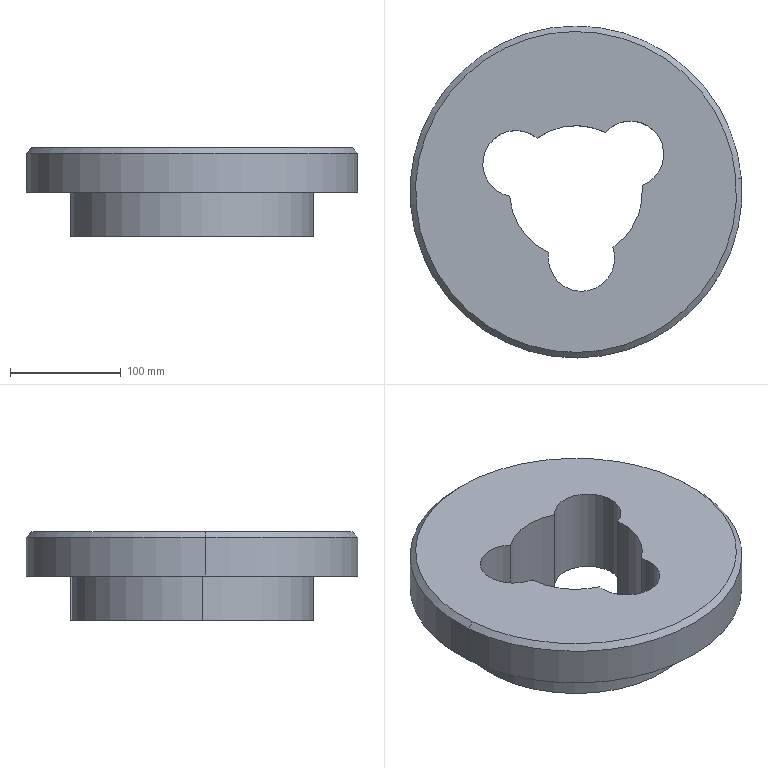Part | SolidWorks | features BaseBody 1 | 1 solid | 25 faces | box 300 x 300 x 80 mm | volume 3048135 mm3 | cylinder 17 | plane 6 | cone 2 | commonest cylinder face diameters 60 x7 120 x5 220 x3 300 x2
STEP:
#1=CARTESIAN_POINT('',(120.577,941.215,-684.893));
#2=VERTEX_POINT('',#1);
#3=CARTESIAN_POINT('',(115.594,940.8,-689.893));
#4=VERTEX_POINT('',#3);
#5=CARTESIAN_POINT('',(115.594,940.8,-689.893));
#6=DIRECTION('',(-0.7047,-0.05869,-0.7071));
#7=VECTOR('',#6,1000.);
#8=LINE('',#5,#7);
#9=EDGE_CURVE('',#2,#4,#8,.T.);
#10=ORIENTED_EDGE('',*,*,#9,.F.);
#11=CARTESIAN_POINT('',(409.577,965.283,-684.893));
#12=VERTEX_POINT('',#11);
#13=CARTESIAN_POINT('',(265.077,953.249,-684.893));
#14=DIRECTION('',(0.,0.,1.));
#15=DIRECTION('',(0.9965,0.083,0.));
#16=AXIS2_PLACEMENT_3D('',#13,#14,#15);
#17=CIRCLE('',#16,145.);
#18=EDGE_CURVE('',#12,#2,#17,.T.);
#19=ORIENTED_EDGE('',*,*,#18,.F.);
#20=CARTESIAN_POINT('',(414.559,965.698,-689.893));
#21=VERTEX_POINT('',#20);
#22=CARTESIAN_POINT('',(414.559,965.698,-689.893));
#23=DIRECTION('',(0.7047,0.05869,-0.7071));
#24=VECTOR('',#23,1000.);
#25=LINE('',#22,#24);
#26=EDGE_CURVE('',#12,#21,#25,.T.);
#27=ORIENTED_EDGE('',*,*,#26,.T.);
#28=CARTESIAN_POINT('',(265.077,953.249,-689.893));
#29=DIRECTION('',(0.,0.,-1.));
#30=DIRECTION('',(0.9965,0.083,0.));
#31=AXIS2_PLACEMENT_3D('',#28,#29,#30);
#32=CIRCLE('',#31,150.);
#33=EDGE_CURVE('',#4,#21,#32,.T.);
#34=ORIENTED_EDGE('',*,*,#33,.F.);
#35=EDGE_LOOP('',(#10,#19,#27,#34));
#36=FACE_OUTER_BOUND('',#35,.T.);
#37=CARTESIAN_POINT('',(265.077,953.249,-689.893));
#38=DIRECTION('',(0.,0.,-1.));
#39=DIRECTION('',(-0.9965,-0.083,0.));
#40=AXIS2_PLACEMENT_3D('',#37,#38,#39);
#41=CONICAL_SURFACE('',#40,150.,0.7854);
#42=ADVANCED_FACE('',(#36),#41,.T.);
#43=CARTESIAN_POINT('',(265.951,1063.245,-724.893));
#44=VERTEX_POINT('',#43);
#45=CARTESIAN_POINT('',(374.697,962.379,-724.893));
#46=VERTEX_POINT('',#45);
#47=CARTESIAN_POINT('',(265.077,953.249,-724.893));
#48=DIRECTION('',(0.,0.,-1.));
#49=DIRECTION('',(0.9965,0.083,0.));
#50=AXIS2_PLACEMENT_3D('',#47,#48,#49);
#51=CIRCLE('',#50,110.);
#52=EDGE_CURVE('',#44,#46,#51,.T.);
#53=ORIENTED_EDGE('',*,*,#52,.F.);
#54=CARTESIAN_POINT('',(266.743,1053.734,-724.893));
#55=VERTEX_POINT('',#54);
#56=CARTESIAN_POINT('',(247.642,1283.081,-724.893));
#57=DIRECTION('',(0.083,-0.9965,0.));
#58=VECTOR('',#57,1000.);
#59=LINE('',#56,#58);
#60=EDGE_CURVE('',#44,#55,#59,.T.);
#61=ORIENTED_EDGE('',*,*,#60,.T.);
#62=CARTESIAN_POINT('',(246.812,1052.074,-724.893));
#63=VERTEX_POINT('',#62);
#64=CARTESIAN_POINT('',(256.777,1052.904,-724.893));
#65=DIRECTION('',(0.9965,0.083,0.));
#66=VECTOR('',#65,1000.);
#67=LINE('',#64,#66);
#68=EDGE_CURVE('',#63,#55,#67,.T.);
#69=ORIENTED_EDGE('',*,*,#68,.F.);
#70=CARTESIAN_POINT('',(246.02,1061.586,-724.893));
#71=VERTEX_POINT('',#70);
#72=CARTESIAN_POINT('',(227.711,1281.421,-724.893));
#73=DIRECTION('',(0.083,-0.9965,0.));
#74=VECTOR('',#73,1000.);
#75=LINE('',#72,#74);
#76=EDGE_CURVE('',#71,#63,#75,.T.);
#77=ORIENTED_EDGE('',*,*,#76,.F.);
#78=CARTESIAN_POINT('',(155.456,944.119,-724.893));
#79=VERTEX_POINT('',#78);
#80=CARTESIAN_POINT('',(265.077,953.249,-724.893));
#81=DIRECTION('',(0.,0.,-1.));
#82=DIRECTION('',(0.9965,0.083,0.));
#83=AXIS2_PLACEMENT_3D('',#80,#81,#82);
#84=CIRCLE('',#83,110.);
#85=EDGE_CURVE('',#79,#71,#84,.T.);
#86=ORIENTED_EDGE('',*,*,#85,.F.);
#87=CARTESIAN_POINT('',(265.077,953.249,-724.893));
#88=DIRECTION('',(0.,0.,-1.));
#89=DIRECTION('',(0.9965,0.083,0.));
#90=AXIS2_PLACEMENT_3D('',#87,#88,#89);
#91=CIRCLE('',#90,110.);
#92=EDGE_CURVE('',#46,#79,#91,.T.);
#93=ORIENTED_EDGE('',*,*,#92,.F.);
#94=EDGE_LOOP('',(#53,#61,#69,#77,#86,#93));
#95=FACE_BOUND('',#94,.T.);
#96=CARTESIAN_POINT('',(414.559,965.698,-724.893));
#97=VERTEX_POINT('',#96);
#98=CARTESIAN_POINT('',(115.594,940.8,-724.893));
#99=VERTEX_POINT('',#98);
#100=CARTESIAN_POINT('',(265.077,953.249,-724.893));
#101=DIRECTION('',(0.,0.,-1.));
#102=DIRECTION('',(0.9965,0.083,0.));
#103=AXIS2_PLACEMENT_3D('',#100,#101,#102);
#104=CIRCLE('',#103,150.);
#105=EDGE_CURVE('',#97,#99,#104,.T.);
#106=ORIENTED_EDGE('',*,*,#105,.T.);
#107=CARTESIAN_POINT('',(265.077,953.249,-724.893));
#108=DIRECTION('',(0.,0.,-1.));
#109=DIRECTION('',(0.9965,0.083,0.));
#110=AXIS2_PLACEMENT_3D('',#107,#108,#109);
#111=CIRCLE('',#110,150.);
#112=EDGE_CURVE('',#99,#97,#111,.T.);
#113=ORIENTED_EDGE('',*,*,#112,.T.);
#114=EDGE_LOOP('',(#106,#113));
#115=FACE_OUTER_BOUND('',#114,.T.);
#116=CARTESIAN_POINT('',(237.676,1282.251,-724.893));
#117=DIRECTION('',(0.,0.,-1.));
#118=DIRECTION('',(0.,-1.,0.));
#119=AXIS2_PLACEMENT_3D('',#116,#117,#118);
#120=PLANE('',#119);
#121=ADVANCED_FACE('',(#95,#115),#120,.T.);
#122=CARTESIAN_POINT('',(324.769,959.318,-684.893));
#123=VERTEX_POINT('',#122);
#124=CARTESIAN_POINT('',(324.87,958.229,-684.893));
#125=VERTEX_POINT('',#124);
#126=CARTESIAN_POINT('',(265.077,953.249,-684.893));
#127=DIRECTION('',(0.,0.,-1.));
#128=DIRECTION('',(0.9965,0.083,0.));
#129=AXIS2_PLACEMENT_3D('',#126,#127,#128);
#130=CIRCLE('',#129,60.);
#131=EDGE_CURVE('',#123,#125,#130,.T.);
#132=ORIENTED_EDGE('',*,*,#131,.T.);
#133=CARTESIAN_POINT('',(298.381,903.341,-684.893));
#134=VERTEX_POINT('',#133);
#135=CARTESIAN_POINT('',(265.077,953.249,-684.893));
#136=DIRECTION('',(0.,0.,-1.));
#137=DIRECTION('',(0.9965,0.083,0.));
#138=AXIS2_PLACEMENT_3D('',#135,#136,#137);
#139=CIRCLE('',#138,60.);
#140=EDGE_CURVE('',#125,#134,#139,.T.);
#141=ORIENTED_EDGE('',*,*,#140,.T.);
#142=CARTESIAN_POINT('',(299.953,895.946,-684.893));
#143=VERTEX_POINT('',#142);
#144=CARTESIAN_POINT('',(270.057,893.456,-684.893));
#145=DIRECTION('',(0.,0.,-1.));
#146=DIRECTION('',(0.9965,0.083,0.));
#147=AXIS2_PLACEMENT_3D('',#144,#145,#146);
#148=CIRCLE('',#147,30.);
#149=EDGE_CURVE('',#134,#143,#148,.T.);
#150=ORIENTED_EDGE('',*,*,#149,.T.);
#151=CARTESIAN_POINT('',(240.16,890.966,-684.893));
#152=VERTEX_POINT('',#151);
#153=CARTESIAN_POINT('',(270.057,893.456,-684.893));
#154=DIRECTION('',(0.,0.,-1.));
#155=DIRECTION('',(0.9965,0.083,0.));
#156=AXIS2_PLACEMENT_3D('',#153,#154,#155);
#157=CIRCLE('',#156,30.);
#158=EDGE_CURVE('',#143,#152,#157,.T.);
#159=ORIENTED_EDGE('',*,*,#158,.T.);
#160=CARTESIAN_POINT('',(240.487,898.519,-684.893));
#161=VERTEX_POINT('',#160);
#162=CARTESIAN_POINT('',(270.057,893.456,-684.893));
#163=DIRECTION('',(0.,0.,-1.));
#164=DIRECTION('',(0.9965,0.083,0.));
#165=AXIS2_PLACEMENT_3D('',#162,#163,#164);
#166=CIRCLE('',#165,30.);
#167=EDGE_CURVE('',#152,#161,#166,.T.);
#168=ORIENTED_EDGE('',*,*,#167,.T.);
#169=CARTESIAN_POINT('',(205.284,948.269,-684.893));
#170=VERTEX_POINT('',#169);
#171=CARTESIAN_POINT('',(265.077,953.249,-684.893));
#172=DIRECTION('',(0.,0.,-1.));
#173=DIRECTION('',(0.9965,0.083,0.));
#174=AXIS2_PLACEMENT_3D('',#171,#172,#173);
#175=CIRCLE('',#174,60.);
#176=EDGE_CURVE('',#161,#170,#175,.T.);
#177=ORIENTED_EDGE('',*,*,#176,.T.);
#178=CARTESIAN_POINT('',(205.203,949.36,-684.893));
#179=VERTEX_POINT('',#178);
#180=CARTESIAN_POINT('',(265.077,953.249,-684.893));
#181=DIRECTION('',(0.,0.,-1.));
#182=DIRECTION('',(0.9965,0.083,0.));
#183=AXIS2_PLACEMENT_3D('',#180,#181,#182);
#184=CIRCLE('',#183,60.);
#185=EDGE_CURVE('',#170,#179,#184,.T.);
#186=ORIENTED_EDGE('',*,*,#185,.T.);
#187=CARTESIAN_POINT('',(180.908,976.343,-684.893));
#188=VERTEX_POINT('',#187);
#189=CARTESIAN_POINT('',(210.805,978.833,-684.893));
#190=DIRECTION('',(0.,0.,-1.));
#191=DIRECTION('',(0.9965,0.083,0.));
#192=AXIS2_PLACEMENT_3D('',#189,#190,#191);
#193=CIRCLE('',#192,30.);
#194=EDGE_CURVE('',#179,#188,#193,.T.);
#195=ORIENTED_EDGE('',*,*,#194,.T.);
#196=CARTESIAN_POINT('',(229.975,1001.909,-684.893));
#197=VERTEX_POINT('',#196);
#198=CARTESIAN_POINT('',(210.805,978.833,-684.893));
#199=DIRECTION('',(0.,0.,-1.));
#200=DIRECTION('',(0.9965,0.083,0.));
#201=AXIS2_PLACEMENT_3D('',#198,#199,#200);
#202=CIRCLE('',#201,30.);
#203=EDGE_CURVE('',#188,#197,#202,.T.);
#204=ORIENTED_EDGE('',*,*,#203,.T.);
#205=CARTESIAN_POINT('',(291.646,1007.045,-684.893));
#206=VERTEX_POINT('',#205);
#207=CARTESIAN_POINT('',(265.077,953.249,-684.893));
#208=DIRECTION('',(0.,0.,-1.));
#209=DIRECTION('',(0.9965,0.083,0.));
#210=AXIS2_PLACEMENT_3D('',#207,#208,#209);
#211=CIRCLE('',#210,60.);
#212=EDGE_CURVE('',#197,#206,#211,.T.);
#213=ORIENTED_EDGE('',*,*,#212,.T.);
#214=CARTESIAN_POINT('',(344.266,989.948,-684.893));
#215=VERTEX_POINT('',#214);
#216=CARTESIAN_POINT('',(314.369,987.458,-684.893));
#217=DIRECTION('',(0.,0.,-1.));
#218=DIRECTION('',(0.9965,0.083,0.));
#219=AXIS2_PLACEMENT_3D('',#216,#217,#218);
#220=CIRCLE('',#219,30.);
#221=EDGE_CURVE('',#206,#215,#220,.T.);
#222=ORIENTED_EDGE('',*,*,#221,.T.);
#223=CARTESIAN_POINT('',(314.369,987.458,-684.893));
#224=DIRECTION('',(0.,0.,-1.));
#225=DIRECTION('',(0.9965,0.083,0.));
#226=AXIS2_PLACEMENT_3D('',#223,#224,#225);
#227=CIRCLE('',#226,30.);
#228=EDGE_CURVE('',#215,#123,#227,.T.);
#229=ORIENTED_EDGE('',*,*,#228,.T.);
#230=EDGE_LOOP('',(#132,#141,#150,#159,#168,#177,#186,#195,#204,#213,#222,#229));
#231=FACE_BOUND('',#230,.T.);
#232=ORIENTED_EDGE('',*,*,#18,.T.);
#233=CARTESIAN_POINT('',(265.077,953.249,-684.893));
#234=DIRECTION('',(0.,0.,1.));
#235=DIRECTION('',(0.9965,0.083,0.));
#236=AXIS2_PLACEMENT_3D('',#233,#234,#235);
#237=CIRCLE('',#236,145.);
#238=EDGE_CURVE('',#2,#12,#237,.T.);
#239=ORIENTED_EDGE('',*,*,#238,.T.);
#240=EDGE_LOOP('',(#232,#239));
#241=FACE_OUTER_BOUND('',#240,.T.);
#242=CARTESIAN_POINT('',(237.676,1282.251,-684.893));
#243=DIRECTION('',(0.,0.,-1.));
#244=DIRECTION('',(0.,-1.,0.));
#245=AXIS2_PLACEMENT_3D('',#242,#243,#244);
#246=PLANE('',#245);
#247=ADVANCED_FACE('',(#231,#241),#246,.F.);
#248=CARTESIAN_POINT('',(115.594,940.8,-684.893));
#249=DIRECTION('',(0.,0.,-1.));
#250=VECTOR('',#249,1000.);
#251=LINE('',#248,#250);
#252=EDGE_CURVE('',#4,#99,#251,.T.);
#253=ORIENTED_EDGE('',*,*,#252,.F.);
#254=ORIENTED_EDGE('',*,*,#33,.T.);
#255=CARTESIAN_POINT('',(414.559,965.698,-684.893));
#256=DIRECTION('',(0.,0.,-1.));
#257=VECTOR('',#256,1000.);
#258=LINE('',#255,#257);
#259=EDGE_CURVE('',#21,#97,#258,.T.);
#260=ORIENTED_EDGE('',*,*,#259,.T.);
#261=ORIENTED_EDGE('',*,*,#112,.F.);
#262=EDGE_LOOP('',(#253,#254,#260,#261));
#263=FACE_OUTER_BOUND('',#262,.T.);
#264=CARTESIAN_POINT('',(265.077,953.249,-684.893));
#265=DIRECTION('',(0.,0.,-1.));
#266=DIRECTION('',(-0.9965,-0.083,0.));
#267=AXIS2_PLACEMENT_3D('',#264,#265,#266);
#268=CYLINDRICAL_SURFACE('',#267,150.);
#269=ADVANCED_FACE('',(#263),#268,.T.);
#270=CARTESIAN_POINT('',(324.769,959.318,-764.893));
#271=VERTEX_POINT('',#270);
#272=CARTESIAN_POINT('',(324.87,958.229,-764.893));
#273=VERTEX_POINT('',#272);
#274=CARTESIAN_POINT('',(265.077,953.249,-764.893));
#275=DIRECTION('',(0.,0.,-1.));
#276=DIRECTION('',(0.9965,0.083,0.));
#277=AXIS2_PLACEMENT_3D('',#274,#275,#276);
#278=CIRCLE('',#277,60.);
#279=EDGE_CURVE('',#271,#273,#278,.T.);
#280=ORIENTED_EDGE('',*,*,#279,.F.);
#281=CARTESIAN_POINT('',(344.266,989.948,-764.893));
#282=VERTEX_POINT('',#281);
#283=CARTESIAN_POINT('',(314.369,987.458,-764.893));
#284=DIRECTION('',(0.,0.,-1.));
#285=DIRECTION('',(0.9965,0.083,0.));
#286=AXIS2_PLACEMENT_3D('',#283,#284,#285);
#287=CIRCLE('',#286,30.);
#288=EDGE_CURVE('',#282,#271,#287,.T.);
#289=ORIENTED_EDGE('',*,*,#288,.F.);
#290=CARTESIAN_POINT('',(291.646,1007.045,-764.893));
#291=VERTEX_POINT('',#290);
#292=CARTESIAN_POINT('',(314.369,987.458,-764.893));
#293=DIRECTION('',(0.,0.,-1.));
#294=DIRECTION('',(0.9965,0.083,0.));
#295=AXIS2_PLACEMENT_3D('',#292,#293,#294);
#296=CIRCLE('',#295,30.);
#297=EDGE_CURVE('',#291,#282,#296,.T.);
#298=ORIENTED_EDGE('',*,*,#297,.F.);
#299=CARTESIAN_POINT('',(229.975,1001.909,-764.893));
#300=VERTEX_POINT('',#299);
#301=CARTESIAN_POINT('',(265.077,953.249,-764.893));
#302=DIRECTION('',(0.,0.,-1.));
#303=DIRECTION('',(0.9965,0.083,0.));
#304=AXIS2_PLACEMENT_3D('',#301,#302,#303);
#305=CIRCLE('',#304,60.);
#306=EDGE_CURVE('',#300,#291,#305,.T.);
#307=ORIENTED_EDGE('',*,*,#306,.F.);
#308=CARTESIAN_POINT('',(180.908,976.343,-764.893));
#309=VERTEX_POINT('',#308);
#310=CARTESIAN_POINT('',(210.805,978.833,-764.893));
#311=DIRECTION('',(0.,0.,-1.));
#312=DIRECTION('',(0.9965,0.083,0.));
#313=AXIS2_PLACEMENT_3D('',#310,#311,#312);
#314=CIRCLE('',#313,30.);
#315=EDGE_CURVE('',#309,#300,#314,.T.);
#316=ORIENTED_EDGE('',*,*,#315,.F.);
#317=CARTESIAN_POINT('',(205.203,949.36,-764.893));
#318=VERTEX_POINT('',#317);
#319=CARTESIAN_POINT('',(210.805,978.833,-764.893));
#320=DIRECTION('',(0.,0.,-1.));
#321=DIRECTION('',(0.9965,0.083,0.));
#322=AXIS2_PLACEMENT_3D('',#319,#320,#321);
#323=CIRCLE('',#322,30.);
#324=EDGE_CURVE('',#318,#309,#323,.T.);
#325=ORIENTED_EDGE('',*,*,#324,.F.);
#326=CARTESIAN_POINT('',(205.284,948.269,-764.893));
#327=VERTEX_POINT('',#326);
#328=CARTESIAN_POINT('',(265.077,953.249,-764.893));
#329=DIRECTION('',(0.,0.,-1.));
#330=DIRECTION('',(0.9965,0.083,0.));
#331=AXIS2_PLACEMENT_3D('',#328,#329,#330);
#332=CIRCLE('',#331,60.);
#333=EDGE_CURVE('',#327,#318,#332,.T.);
#334=ORIENTED_EDGE('',*,*,#333,.F.);
#335=CARTESIAN_POINT('',(240.487,898.519,-764.893));
#336=VERTEX_POINT('',#335);
#337=CARTESIAN_POINT('',(265.077,953.249,-764.893));
#338=DIRECTION('',(0.,0.,-1.));
#339=DIRECTION('',(0.9965,0.083,0.));
#340=AXIS2_PLACEMENT_3D('',#337,#338,#339);
#341=CIRCLE('',#340,60.);
#342=EDGE_CURVE('',#336,#327,#341,.T.);
#343=ORIENTED_EDGE('',*,*,#342,.F.);
#344=CARTESIAN_POINT('',(240.16,890.966,-764.893));
#345=VERTEX_POINT('',#344);
#346=CARTESIAN_POINT('',(270.057,893.456,-764.893));
#347=DIRECTION('',(0.,0.,-1.));
#348=DIRECTION('',(0.9965,0.083,0.));
#349=AXIS2_PLACEMENT_3D('',#346,#347,#348);
#350=CIRCLE('',#349,30.);
#351=EDGE_CURVE('',#345,#336,#350,.T.);
#352=ORIENTED_EDGE('',*,*,#351,.F.);
#353=CARTESIAN_POINT('',(299.953,895.946,-764.893));
#354=VERTEX_POINT('',#353);
#355=CARTESIAN_POINT('',(270.057,893.456,-764.893));
#356=DIRECTION('',(0.,0.,-1.));
#357=DIRECTION('',(0.9965,0.083,0.));
#358=AXIS2_PLACEMENT_3D('',#355,#356,#357);
#359=CIRCLE('',#358,30.);
#360=EDGE_CURVE('',#354,#345,#359,.T.);
#361=ORIENTED_EDGE('',*,*,#360,.F.);
#362=CARTESIAN_POINT('',(298.381,903.341,-764.893));
#363=VERTEX_POINT('',#362);
#364=CARTESIAN_POINT('',(270.057,893.456,-764.893));
#365=DIRECTION('',(0.,0.,-1.));
#366=DIRECTION('',(0.9965,0.083,0.));
#367=AXIS2_PLACEMENT_3D('',#364,#365,#366);
#368=CIRCLE('',#367,30.);
#369=EDGE_CURVE('',#363,#354,#368,.T.);
#370=ORIENTED_EDGE('',*,*,#369,.F.);
#371=CARTESIAN_POINT('',(265.077,953.249,-764.893));
#372=DIRECTION('',(0.,0.,-1.));
#373=DIRECTION('',(0.9965,0.083,0.));
#374=AXIS2_PLACEMENT_3D('',#371,#372,#373);
#375=CIRCLE('',#374,60.);
#376=EDGE_CURVE('',#273,#363,#375,.T.);
#377=ORIENTED_EDGE('',*,*,#376,.F.);
#378=EDGE_LOOP('',(#280,#289,#298,#307,#316,#325,#334,#343,#352,#361,#370,#377));
#379=FACE_BOUND('',#378,.T.);
#380=CARTESIAN_POINT('',(265.951,1063.245,-764.893));
#381=VERTEX_POINT('',#380);
#382=CARTESIAN_POINT('',(266.743,1053.734,-764.893));
#383=VERTEX_POINT('',#382);
#384=CARTESIAN_POINT('',(247.642,1283.081,-764.893));
#385=DIRECTION('',(0.083,-0.9965,0.));
#386=VECTOR('',#385,1000.);
#387=LINE('',#384,#386);
#388=EDGE_CURVE('',#381,#383,#387,.T.);
#389=ORIENTED_EDGE('',*,*,#388,.F.);
#390=CARTESIAN_POINT('',(374.697,962.379,-764.893));
#391=VERTEX_POINT('',#390);
#392=CARTESIAN_POINT('',(265.077,953.249,-764.893));
#393=DIRECTION('',(0.,0.,-1.));
#394=DIRECTION('',(0.9965,0.083,0.));
#395=AXIS2_PLACEMENT_3D('',#392,#393,#394);
#396=CIRCLE('',#395,110.);
#397=EDGE_CURVE('',#381,#391,#396,.T.);
#398=ORIENTED_EDGE('',*,*,#397,.T.);
#399=CARTESIAN_POINT('',(155.456,944.119,-764.893));
#400=VERTEX_POINT('',#399);
#401=CARTESIAN_POINT('',(265.077,953.249,-764.893));
#402=DIRECTION('',(0.,0.,-1.));
#403=DIRECTION('',(0.9965,0.083,0.));
#404=AXIS2_PLACEMENT_3D('',#401,#402,#403);
#405=CIRCLE('',#404,110.);
#406=EDGE_CURVE('',#391,#400,#405,.T.);
#407=ORIENTED_EDGE('',*,*,#406,.T.);
#408=CARTESIAN_POINT('',(246.02,1061.586,-764.893));
#409=VERTEX_POINT('',#408);
#410=CARTESIAN_POINT('',(265.077,953.249,-764.893));
#411=DIRECTION('',(0.,0.,-1.));
#412=DIRECTION('',(0.9965,0.083,0.));
#413=AXIS2_PLACEMENT_3D('',#410,#411,#412);
#414=CIRCLE('',#413,110.);
#415=EDGE_CURVE('',#400,#409,#414,.T.);
#416=ORIENTED_EDGE('',*,*,#415,.T.);
#417=CARTESIAN_POINT('',(246.812,1052.074,-764.893));
#418=VERTEX_POINT('',#417);
#419=CARTESIAN_POINT('',(227.711,1281.421,-764.893));
#420=DIRECTION('',(0.083,-0.9965,0.));
#421=VECTOR('',#420,1000.);
#422=LINE('',#419,#421);
#423=EDGE_CURVE('',#409,#418,#422,.T.);
#424=ORIENTED_EDGE('',*,*,#423,.T.);
#425=CARTESIAN_POINT('',(256.777,1052.904,-764.893));
#426=DIRECTION('',(0.9965,0.083,0.));
#427=VECTOR('',#426,1000.);
#428=LINE('',#425,#427);
#429=EDGE_CURVE('',#418,#383,#428,.T.);
#430=ORIENTED_EDGE('',*,*,#429,.T.);
#431=EDGE_LOOP('',(#389,#398,#407,#416,#424,#430));
#432=FACE_OUTER_BOUND('',#431,.T.);
#433=CARTESIAN_POINT('',(237.676,1282.251,-764.893));
#434=DIRECTION('',(0.,0.,-1.));
#435=DIRECTION('',(0.,-1.,0.));
#436=AXIS2_PLACEMENT_3D('',#433,#434,#435);
#437=PLANE('',#436);
#438=ADVANCED_FACE('',(#379,#432),#437,.T.);
#439=ORIENTED_EDGE('',*,*,#68,.T.);
#440=CARTESIAN_POINT('',(266.743,1053.734,-764.893));
#441=DIRECTION('',(0.,0.,1.));
#442=VECTOR('',#441,1000.);
#443=LINE('',#440,#442);
#444=EDGE_CURVE('',#383,#55,#443,.T.);
#445=ORIENTED_EDGE('',*,*,#444,.F.);
#446=ORIENTED_EDGE('',*,*,#429,.F.);
#447=CARTESIAN_POINT('',(246.812,1052.074,-764.893));
#448=DIRECTION('',(0.,0.,1.));
#449=VECTOR('',#448,1000.);
#450=LINE('',#447,#449);
#451=EDGE_CURVE('',#418,#63,#450,.T.);
#452=ORIENTED_EDGE('',*,*,#451,.T.);
#453=EDGE_LOOP('',(#439,#445,#446,#452));
#454=FACE_OUTER_BOUND('',#453,.T.);
#455=CARTESIAN_POINT('',(256.777,1052.904,-764.893));
#456=DIRECTION('',(0.083,-0.9965,0.));
#457=DIRECTION('',(0.,0.,-1.));
#458=AXIS2_PLACEMENT_3D('',#455,#456,#457);
#459=PLANE('',#458);
#460=ADVANCED_FACE('',(#454),#459,.F.);
#461=CARTESIAN_POINT('',(240.16,890.966,-764.893));
#462=DIRECTION('',(0.,0.,1.));
#463=VECTOR('',#462,1000.);
#464=LINE('',#461,#463);
#465=EDGE_CURVE('',#345,#152,#464,.T.);
#466=ORIENTED_EDGE('',*,*,#465,.F.);
#467=ORIENTED_EDGE('',*,*,#351,.T.);
#468=CARTESIAN_POINT('',(240.487,898.519,-764.893));
#469=DIRECTION('',(0.,0.,1.));
#470=VECTOR('',#469,1000.);
#471=LINE('',#468,#470);
#472=EDGE_CURVE('',#336,#161,#471,.T.);
#473=ORIENTED_EDGE('',*,*,#472,.T.);
#474=ORIENTED_EDGE('',*,*,#167,.F.);
#475=EDGE_LOOP('',(#466,#467,#473,#474));
#476=FACE_OUTER_BOUND('',#475,.T.);
#477=CARTESIAN_POINT('',(270.057,893.456,-764.893));
#478=DIRECTION('',(0.,0.,1.));
#479=DIRECTION('',(0.9965,0.083,0.));
#480=AXIS2_PLACEMENT_3D('',#477,#478,#479);
#481=CYLINDRICAL_SURFACE('',#480,30.);
#482=ADVANCED_FACE('',(#476),#481,.F.);
#483=CARTESIAN_POINT('',(205.284,948.269,-764.893));
#484=DIRECTION('',(0.,0.,1.));
#485=VECTOR('',#484,1000.);
#486=LINE('',#483,#485);
#487=EDGE_CURVE('',#327,#170,#486,.T.);
#488=ORIENTED_EDGE('',*,*,#487,.F.);
#489=ORIENTED_EDGE('',*,*,#333,.T.);
#490=CARTESIAN_POINT('',(205.203,949.36,-764.893));
#491=DIRECTION('',(0.,0.,1.));
#492=VECTOR('',#491,1000.);
#493=LINE('',#490,#492);
#494=EDGE_CURVE('',#318,#179,#493,.T.);
#495=ORIENTED_EDGE('',*,*,#494,.T.);
#496=ORIENTED_EDGE('',*,*,#185,.F.);
#497=EDGE_LOOP('',(#488,#489,#495,#496));
#498=FACE_OUTER_BOUND('',#497,.T.);
#499=CARTESIAN_POINT('',(265.077,953.249,-764.893));
#500=DIRECTION('',(0.,0.,1.));
#501=DIRECTION('',(0.9965,0.083,0.));
#502=AXIS2_PLACEMENT_3D('',#499,#500,#501);
#503=CYLINDRICAL_SURFACE('',#502,60.);
#504=ADVANCED_FACE('',(#498),#503,.F.);
#505=CARTESIAN_POINT('',(180.908,976.343,-764.893));
#506=DIRECTION('',(0.,0.,1.));
#507=VECTOR('',#506,1000.);
#508=LINE('',#505,#507);
#509=EDGE_CURVE('',#309,#188,#508,.T.);
#510=ORIENTED_EDGE('',*,*,#509,.F.);
#511=ORIENTED_EDGE('',*,*,#315,.T.);
#512=CARTESIAN_POINT('',(229.975,1001.909,-764.893));
#513=DIRECTION('',(0.,0.,1.));
#514=VECTOR('',#513,1000.);
#515=LINE('',#512,#514);
#516=EDGE_CURVE('',#300,#197,#515,.T.);
#517=ORIENTED_EDGE('',*,*,#516,.T.);
#518=ORIENTED_EDGE('',*,*,#203,.F.);
#519=EDGE_LOOP('',(#510,#511,#517,#518));
#520=FACE_OUTER_BOUND('',#519,.T.);
#521=CARTESIAN_POINT('',(210.805,978.833,-764.893));
#522=DIRECTION('',(0.,0.,1.));
#523=DIRECTION('',(0.9965,0.083,0.));
#524=AXIS2_PLACEMENT_3D('',#521,#522,#523);
#525=CYLINDRICAL_SURFACE('',#524,30.);
#526=ADVANCED_FACE('',(#520),#525,.F.);
#527=CARTESIAN_POINT('',(291.646,1007.045,-764.893));
#528=DIRECTION('',(0.,0.,1.));
#529=VECTOR('',#528,1000.);
#530=LINE('',#527,#529);
#531=EDGE_CURVE('',#291,#206,#530,.T.);
#532=ORIENTED_EDGE('',*,*,#531,.T.);
#533=ORIENTED_EDGE('',*,*,#212,.F.);
#534=ORIENTED_EDGE('',*,*,#516,.F.);
#535=ORIENTED_EDGE('',*,*,#306,.T.);
#536=EDGE_LOOP('',(#532,#533,#534,#535));
#537=FACE_OUTER_BOUND('',#536,.T.);
#538=CARTESIAN_POINT('',(265.077,953.249,-764.893));
#539=DIRECTION('',(0.,0.,1.));
#540=DIRECTION('',(0.9965,0.083,0.));
#541=AXIS2_PLACEMENT_3D('',#538,#539,#540);
#542=CYLINDRICAL_SURFACE('',#541,60.);
#543=ADVANCED_FACE('',(#537),#542,.F.);
#544=CARTESIAN_POINT('',(344.266,989.948,-764.893));
#545=DIRECTION('',(0.,0.,1.));
#546=VECTOR('',#545,1000.);
#547=LINE('',#544,#546);
#548=EDGE_CURVE('',#282,#215,#547,.T.);
#549=ORIENTED_EDGE('',*,*,#548,.F.);
#550=ORIENTED_EDGE('',*,*,#288,.T.);
#551=CARTESIAN_POINT('',(324.769,959.318,-764.893));
#552=DIRECTION('',(0.,0.,1.));
#553=VECTOR('',#552,1000.);
#554=LINE('',#551,#553);
#555=EDGE_CURVE('',#271,#123,#554,.T.);
#556=ORIENTED_EDGE('',*,*,#555,.T.);
#557=ORIENTED_EDGE('',*,*,#228,.F.);
#558=EDGE_LOOP('',(#549,#550,#556,#557));
#559=FACE_OUTER_BOUND('',#558,.T.);
#560=CARTESIAN_POINT('',(314.369,987.458,-764.893));
#561=DIRECTION('',(0.,0.,1.));
#562=DIRECTION('',(0.9965,0.083,0.));
#563=AXIS2_PLACEMENT_3D('',#560,#561,#562);
#564=CYLINDRICAL_SURFACE('',#563,30.);
#565=ADVANCED_FACE('',(#559),#564,.F.);
#566=CARTESIAN_POINT('',(324.87,958.229,-764.893));
#567=DIRECTION('',(0.,0.,1.));
#568=VECTOR('',#567,1000.);
#569=LINE('',#566,#568);
#570=EDGE_CURVE('',#273,#125,#569,.T.);
#571=ORIENTED_EDGE('',*,*,#570,.F.);
#572=ORIENTED_EDGE('',*,*,#376,.T.);
#573=CARTESIAN_POINT('',(298.381,903.341,-764.893));
#574=DIRECTION('',(0.,0.,1.));
#575=VECTOR('',#574,1000.);
#576=LINE('',#573,#575);
#577=EDGE_CURVE('',#363,#134,#576,.T.);
#578=ORIENTED_EDGE('',*,*,#577,.T.);
#579=ORIENTED_EDGE('',*,*,#140,.F.);
#580=EDGE_LOOP('',(#571,#572,#578,#579));
#581=FACE_OUTER_BOUND('',#580,.T.);
#582=CARTESIAN_POINT('',(265.077,953.249,-764.893));
#583=DIRECTION('',(0.,0.,1.));
#584=DIRECTION('',(0.9965,0.083,0.));
#585=AXIS2_PLACEMENT_3D('',#582,#583,#584);
#586=CYLINDRICAL_SURFACE('',#585,60.);
#587=ADVANCED_FACE('',(#581),#586,.F.);
#588=ORIENTED_EDGE('',*,*,#76,.T.);
#589=ORIENTED_EDGE('',*,*,#451,.F.);
#590=ORIENTED_EDGE('',*,*,#423,.F.);
#591=CARTESIAN_POINT('',(246.02,1061.586,-764.893));
#592=DIRECTION('',(0.,0.,1.));
#593=VECTOR('',#592,1000.);
#594=LINE('',#591,#593);
#595=EDGE_CURVE('',#409,#71,#594,.T.);
#596=ORIENTED_EDGE('',*,*,#595,.T.);
#597=EDGE_LOOP('',(#588,#589,#590,#596));
#598=FACE_OUTER_BOUND('',#597,.T.);
#599=CARTESIAN_POINT('',(227.711,1281.421,-764.893));
#600=DIRECTION('',(-0.9965,-0.083,0.));
#601=DIRECTION('',(-0.083,0.9965,0.));
#602=AXIS2_PLACEMENT_3D('',#599,#600,#601);
#603=PLANE('',#602);
#604=ADVANCED_FACE('',(#598),#603,.F.);
#605=CARTESIAN_POINT('',(374.697,962.379,-764.893));
#606=DIRECTION('',(0.,0.,1.));
#607=VECTOR('',#606,1000.);
#608=LINE('',#605,#607);
#609=EDGE_CURVE('',#391,#46,#608,.T.);
#610=ORIENTED_EDGE('',*,*,#609,.F.);
#611=ORIENTED_EDGE('',*,*,#397,.F.);
#612=CARTESIAN_POINT('',(265.951,1063.245,-764.893));
#613=DIRECTION('',(0.,0.,1.));
#614=VECTOR('',#613,1000.);
#615=LINE('',#612,#614);
#616=EDGE_CURVE('',#381,#44,#615,.T.);
#617=ORIENTED_EDGE('',*,*,#616,.T.);
#618=ORIENTED_EDGE('',*,*,#52,.T.);
#619=EDGE_LOOP('',(#610,#611,#617,#618));
#620=FACE_OUTER_BOUND('',#619,.T.);
#621=CARTESIAN_POINT('',(265.077,953.249,-764.893));
#622=DIRECTION('',(0.,0.,1.));
#623=DIRECTION('',(0.9965,0.083,0.));
#624=AXIS2_PLACEMENT_3D('',#621,#622,#623);
#625=CYLINDRICAL_SURFACE('',#624,110.);
#626=ADVANCED_FACE('',(#620),#625,.T.);
#627=ORIENTED_EDGE('',*,*,#60,.F.);
#628=ORIENTED_EDGE('',*,*,#616,.F.);
#629=ORIENTED_EDGE('',*,*,#388,.T.);
#630=ORIENTED_EDGE('',*,*,#444,.T.);
#631=EDGE_LOOP('',(#627,#628,#629,#630));
#632=FACE_OUTER_BOUND('',#631,.T.);
#633=CARTESIAN_POINT('',(247.642,1283.081,-764.893));
#634=DIRECTION('',(-0.9965,-0.083,0.));
#635=DIRECTION('',(-0.083,0.9965,0.));
#636=AXIS2_PLACEMENT_3D('',#633,#634,#635);
#637=PLANE('',#636);
#638=ADVANCED_FACE('',(#632),#637,.T.);
#639=ORIENTED_EDGE('',*,*,#415,.F.);
#640=CARTESIAN_POINT('',(155.456,944.119,-764.893));
#641=DIRECTION('',(0.,0.,1.));
#642=VECTOR('',#641,1000.);
#643=LINE('',#640,#642);
#644=EDGE_CURVE('',#400,#79,#643,.T.);
#645=ORIENTED_EDGE('',*,*,#644,.T.);
#646=ORIENTED_EDGE('',*,*,#85,.T.);
#647=ORIENTED_EDGE('',*,*,#595,.F.);
#648=EDGE_LOOP('',(#639,#645,#646,#647));
#649=FACE_OUTER_BOUND('',#648,.T.);
#650=CARTESIAN_POINT('',(265.077,953.249,-764.893));
#651=DIRECTION('',(0.,0.,1.));
#652=DIRECTION('',(0.9965,0.083,0.));
#653=AXIS2_PLACEMENT_3D('',#650,#651,#652);
#654=CYLINDRICAL_SURFACE('',#653,110.);
#655=ADVANCED_FACE('',(#649),#654,.T.);
#656=ORIENTED_EDGE('',*,*,#406,.F.);
#657=ORIENTED_EDGE('',*,*,#609,.T.);
#658=ORIENTED_EDGE('',*,*,#92,.T.);
#659=ORIENTED_EDGE('',*,*,#644,.F.);
#660=EDGE_LOOP('',(#656,#657,#658,#659));
#661=FACE_OUTER_BOUND('',#660,.T.);
#662=CARTESIAN_POINT('',(265.077,953.249,-764.893));
#663=DIRECTION('',(0.,0.,1.));
#664=DIRECTION('',(0.9965,0.083,0.));
#665=AXIS2_PLACEMENT_3D('',#662,#663,#664);
#666=CYLINDRICAL_SURFACE('',#665,110.);
#667=ADVANCED_FACE('',(#661),#666,.T.);
#668=ORIENTED_EDGE('',*,*,#324,.T.);
#669=ORIENTED_EDGE('',*,*,#509,.T.);
#670=ORIENTED_EDGE('',*,*,#194,.F.);
#671=ORIENTED_EDGE('',*,*,#494,.F.);
#672=EDGE_LOOP('',(#668,#669,#670,#671));
#673=FACE_OUTER_BOUND('',#672,.T.);
#674=CARTESIAN_POINT('',(210.805,978.833,-764.893));
#675=DIRECTION('',(0.,0.,1.));
#676=DIRECTION('',(0.9965,0.083,0.));
#677=AXIS2_PLACEMENT_3D('',#674,#675,#676);
#678=CYLINDRICAL_SURFACE('',#677,30.);
#679=ADVANCED_FACE('',(#673),#678,.F.);
#680=ORIENTED_EDGE('',*,*,#342,.T.);
#681=ORIENTED_EDGE('',*,*,#487,.T.);
#682=ORIENTED_EDGE('',*,*,#176,.F.);
#683=ORIENTED_EDGE('',*,*,#472,.F.);
#684=EDGE_LOOP('',(#680,#681,#682,#683));
#685=FACE_OUTER_BOUND('',#684,.T.);
#686=CARTESIAN_POINT('',(265.077,953.249,-764.893));
#687=DIRECTION('',(0.,0.,1.));
#688=DIRECTION('',(0.9965,0.083,0.));
#689=AXIS2_PLACEMENT_3D('',#686,#687,#688);
#690=CYLINDRICAL_SURFACE('',#689,60.);
#691=ADVANCED_FACE('',(#685),#690,.F.);
#692=CARTESIAN_POINT('',(299.953,895.946,-764.893));
#693=DIRECTION('',(0.,0.,1.));
#694=VECTOR('',#693,1000.);
#695=LINE('',#692,#694);
#696=EDGE_CURVE('',#354,#143,#695,.T.);
#697=ORIENTED_EDGE('',*,*,#696,.F.);
#698=ORIENTED_EDGE('',*,*,#360,.T.);
#699=ORIENTED_EDGE('',*,*,#465,.T.);
#700=ORIENTED_EDGE('',*,*,#158,.F.);
#701=EDGE_LOOP('',(#697,#698,#699,#700));
#702=FACE_OUTER_BOUND('',#701,.T.);
#703=CARTESIAN_POINT('',(270.057,893.456,-764.893));
#704=DIRECTION('',(0.,0.,1.));
#705=DIRECTION('',(0.9965,0.083,0.));
#706=AXIS2_PLACEMENT_3D('',#703,#704,#705);
#707=CYLINDRICAL_SURFACE('',#706,30.);
#708=ADVANCED_FACE('',(#702),#707,.F.);
#709=ORIENTED_EDGE('',*,*,#369,.T.);
#710=ORIENTED_EDGE('',*,*,#696,.T.);
#711=ORIENTED_EDGE('',*,*,#149,.F.);
#712=ORIENTED_EDGE('',*,*,#577,.F.);
#713=EDGE_LOOP('',(#709,#710,#711,#712));
#714=FACE_OUTER_BOUND('',#713,.T.);
#715=CARTESIAN_POINT('',(270.057,893.456,-764.893));
#716=DIRECTION('',(0.,0.,1.));
#717=DIRECTION('',(0.9965,0.083,0.));
#718=AXIS2_PLACEMENT_3D('',#715,#716,#717);
#719=CYLINDRICAL_SURFACE('',#718,30.);
#720=ADVANCED_FACE('',(#714),#719,.F.);
#721=CARTESIAN_POINT('',(265.077,953.249,-689.893));
#722=DIRECTION('',(0.,0.,-1.));
#723=DIRECTION('',(0.9965,0.083,0.));
#724=AXIS2_PLACEMENT_3D('',#721,#722,#723);
#725=CIRCLE('',#724,150.);
#726=EDGE_CURVE('',#21,#4,#725,.T.);
#727=ORIENTED_EDGE('',*,*,#726,.T.);
#728=ORIENTED_EDGE('',*,*,#252,.T.);
#729=ORIENTED_EDGE('',*,*,#105,.F.);
#730=ORIENTED_EDGE('',*,*,#259,.F.);
#731=EDGE_LOOP('',(#727,#728,#729,#730));
#732=FACE_OUTER_BOUND('',#731,.T.);
#733=CARTESIAN_POINT('',(265.077,953.249,-684.893));
#734=DIRECTION('',(0.,0.,-1.));
#735=DIRECTION('',(-0.9965,-0.083,0.));
#736=AXIS2_PLACEMENT_3D('',#733,#734,#735);
#737=CYLINDRICAL_SURFACE('',#736,150.);
#738=ADVANCED_FACE('',(#732),#737,.T.);
#739=ORIENTED_EDGE('',*,*,#238,.F.);
#740=ORIENTED_EDGE('',*,*,#9,.T.);
#741=ORIENTED_EDGE('',*,*,#726,.F.);
#742=ORIENTED_EDGE('',*,*,#26,.F.);
#743=EDGE_LOOP('',(#739,#740,#741,#742));
#744=FACE_OUTER_BOUND('',#743,.T.);
#745=CARTESIAN_POINT('',(265.077,953.249,-689.893));
#746=DIRECTION('',(0.,0.,-1.));
#747=DIRECTION('',(-0.9965,-0.083,0.));
#748=AXIS2_PLACEMENT_3D('',#745,#746,#747);
#749=CONICAL_SURFACE('',#748,150.,0.7854);
#750=ADVANCED_FACE('',(#744),#749,.T.);
#751=ORIENTED_EDGE('',*,*,#279,.T.);
#752=ORIENTED_EDGE('',*,*,#570,.T.);
#753=ORIENTED_EDGE('',*,*,#131,.F.);
#754=ORIENTED_EDGE('',*,*,#555,.F.);
#755=EDGE_LOOP('',(#751,#752,#753,#754));
#756=FACE_OUTER_BOUND('',#755,.T.);
#757=CARTESIAN_POINT('',(265.077,953.249,-764.893));
#758=DIRECTION('',(0.,0.,1.));
#759=DIRECTION('',(0.9965,0.083,0.));
#760=AXIS2_PLACEMENT_3D('',#757,#758,#759);
#761=CYLINDRICAL_SURFACE('',#760,60.);
#762=ADVANCED_FACE('',(#756),#761,.F.);
#763=ORIENTED_EDGE('',*,*,#297,.T.);
#764=ORIENTED_EDGE('',*,*,#548,.T.);
#765=ORIENTED_EDGE('',*,*,#221,.F.);
#766=ORIENTED_EDGE('',*,*,#531,.F.);
#767=EDGE_LOOP('',(#763,#764,#765,#766));
#768=FACE_OUTER_BOUND('',#767,.T.);
#769=CARTESIAN_POINT('',(314.369,987.458,-764.893));
#770=DIRECTION('',(0.,0.,1.));
#771=DIRECTION('',(0.9965,0.083,0.));
#772=AXIS2_PLACEMENT_3D('',#769,#770,#771);
#773=CYLINDRICAL_SURFACE('',#772,30.);
#774=ADVANCED_FACE('',(#768),#773,.F.);
#775=CLOSED_SHELL('',(#42,#121,#247,#269,#438,#460,#482,#504,#526,#543,#565,#587,#604,#626,#638,#655,#667,#679,#691,#708,#720,#738,#750,#762,#774));
#776=MANIFOLD_SOLID_BREP('',#775);
#777=CARTESIAN_POINT('',(0.,0.,0.));
#778=DIRECTION('',(0.,0.,1.));
#779=DIRECTION('',(1.,0.,0.));
#780=AXIS2_PLACEMENT_3D('',#777,#778,#779);
#781=(LENGTH_UNIT()NAMED_UNIT(*)SI_UNIT(.MILLI.,.METRE.));
#782=UNCERTAINTY_MEASURE_WITH_UNIT(LENGTH_MEASURE(0.00001),#781,'','');
#783=(NAMED_UNIT(*)PLANE_ANGLE_UNIT()SI_UNIT($,.RADIAN.));
#784=(NAMED_UNIT(*)SI_UNIT($,.STERADIAN.)SOLID_ANGLE_UNIT());
#785=(GEOMETRIC_REPRESENTATION_CONTEXT(3)GLOBAL_UNCERTAINTY_ASSIGNED_CONTEXT((#782))GLOBAL_UNIT_ASSIGNED_CONTEXT((#781,#783,#784))REPRESENTATION_CONTEXT('',''));
#786=ADVANCED_BREP_SHAPE_REPRESENTATION('',(#776,#780),#785);